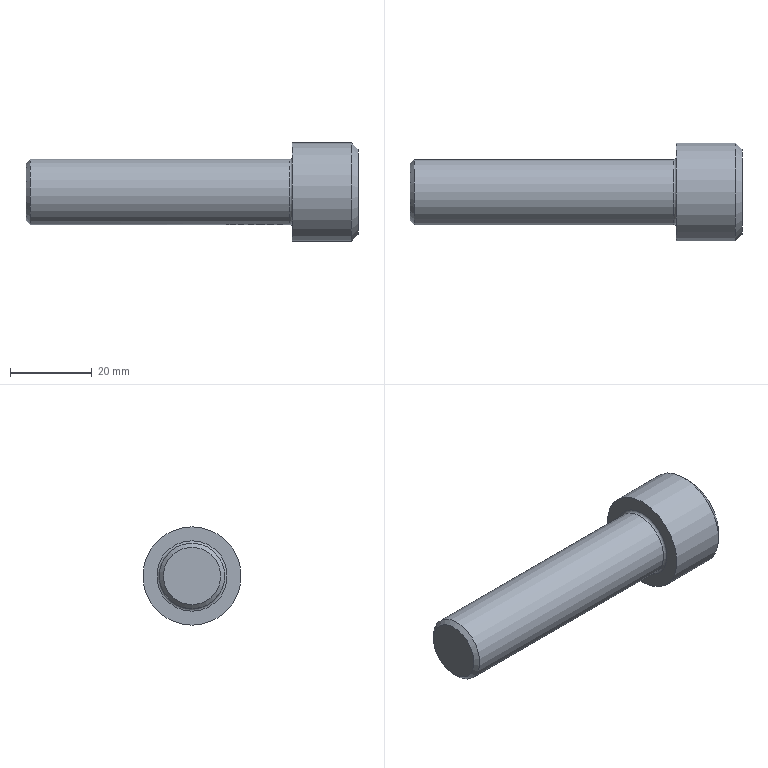Part | STEP file | solid 134 | 1 solid | 111 faces | box 81 x 24 x 24 mm | volume 18829 mm3 | plane 60 | other 35 | cylinder 7 | sphere 6 | cone 2 | torus 1 | commonest cylinder face diameters 16 x6 24 x1